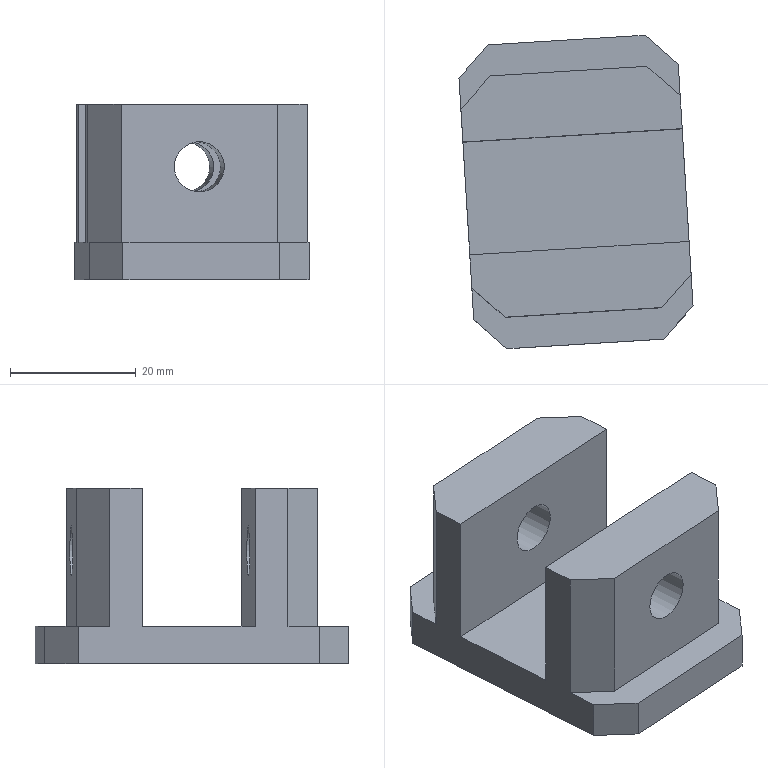Part | STEP file | 车灯-后视镜_id586_x_t | 1 solid | 24 faces | box 37.285 x 49.936 x 28 mm | volume 23540 mm3 | plane 22 | cylinder 2 | commonest cylinder face diameters 8 x2
STEP:
#1=CARTESIAN_POINT('',(116.538,2.661,-249.5));
#2=VERTEX_POINT('',#1);
#3=CARTESIAN_POINT('',(115.439,20.627,-249.5));
#4=VERTEX_POINT('',#3);
#5=CARTESIAN_POINT('',(117.102,-6.572,-249.5));
#6=DIRECTION('',(-0.06105,0.9981,0.));
#7=VECTOR('',#6,1.);
#8=LINE('',#5,#7);
#9=EDGE_CURVE('',#2,#4,#8,.T.);
#10=ORIENTED_EDGE('',*,*,#9,.T.);
#11=CARTESIAN_POINT('',(80.504,18.49,-249.5));
#12=VERTEX_POINT('',#11);
#13=CARTESIAN_POINT('',(103.493,19.896,-249.5));
#14=DIRECTION('',(0.9981,0.06105,0.));
#15=VECTOR('',#14,1.);
#16=LINE('',#13,#15);
#17=EDGE_CURVE('',#12,#4,#16,.T.);
#18=ORIENTED_EDGE('',*,*,#17,.F.);
#19=CARTESIAN_POINT('',(81.603,0.5239,-249.5));
#20=VERTEX_POINT('',#19);
#21=CARTESIAN_POINT('',(82.168,-8.709,-249.5));
#22=DIRECTION('',(0.06105,-0.9981,0.));
#23=VECTOR('',#22,1.);
#24=LINE('',#21,#23);
#25=EDGE_CURVE('',#12,#20,#24,.T.);
#26=ORIENTED_EDGE('',*,*,#25,.T.);
#27=CARTESIAN_POINT('',(104.591,1.93,-249.5));
#28=DIRECTION('',(-0.9981,-0.06105,0.));
#29=VECTOR('',#28,1.);
#30=LINE('',#27,#29);
#31=EDGE_CURVE('',#2,#20,#30,.T.);
#32=ORIENTED_EDGE('',*,*,#31,.F.);
#33=EDGE_LOOP('',(#10,#18,#26,#32));
#34=FACE_OUTER_BOUND('',#33,.T.);
#35=CARTESIAN_POINT('',(111.919,-6.889,-249.5));
#36=DIRECTION('',(0.,0.,1.));
#37=DIRECTION('',(-0.9981,-0.06105,0.));
#38=AXIS2_PLACEMENT_3D('',#35,#36,#37);
#39=PLANE('',#38);
#40=ADVANCED_FACE('',(#34),#39,.T.);
#41=CARTESIAN_POINT('',(117.163,-7.57,-249.5));
#42=VERTEX_POINT('',#41);
#43=CARTESIAN_POINT('',(116.858,-2.58,-249.5));
#44=VERTEX_POINT('',#43);
#45=CARTESIAN_POINT('',(116.4,4.906,-249.5));
#46=DIRECTION('',(-0.06105,0.9981,0.));
#47=VECTOR('',#46,1.);
#48=LINE('',#45,#47);
#49=EDGE_CURVE('',#42,#44,#48,.T.);
#50=ORIENTED_EDGE('',*,*,#49,.T.);
#51=CARTESIAN_POINT('',(112.173,-7.876,-249.5));
#52=VERTEX_POINT('',#51);
#53=CARTESIAN_POINT('',(116.858,-2.58,-249.5));
#54=DIRECTION('',(0.6626,0.749,0.));
#55=VECTOR('',#54,1.);
#56=LINE('',#53,#55);
#57=EDGE_CURVE('',#52,#44,#56,.T.);
#58=ORIENTED_EDGE('',*,*,#57,.F.);
#59=CARTESIAN_POINT('',(87.219,-9.402,-249.5));
#60=VERTEX_POINT('',#59);
#61=CARTESIAN_POINT('',(100.554,-8.586,-249.5));
#62=DIRECTION('',(0.9981,0.06105,0.));
#63=VECTOR('',#62,1.);
#64=LINE('',#61,#63);
#65=EDGE_CURVE('',#60,#52,#64,.T.);
#66=ORIENTED_EDGE('',*,*,#65,.F.);
#67=CARTESIAN_POINT('',(81.923,-4.716,-249.5));
#68=VERTEX_POINT('',#67);
#69=CARTESIAN_POINT('',(87.219,-9.402,-249.5));
#70=DIRECTION('',(0.749,-0.6626,0.));
#71=VECTOR('',#70,1.);
#72=LINE('',#69,#71);
#73=EDGE_CURVE('',#68,#60,#72,.T.);
#74=ORIENTED_EDGE('',*,*,#73,.F.);
#75=CARTESIAN_POINT('',(82.229,-9.707,-249.5));
#76=VERTEX_POINT('',#75);
#77=CARTESIAN_POINT('',(81.466,2.77,-249.5));
#78=DIRECTION('',(0.06105,-0.9981,0.));
#79=VECTOR('',#78,1.);
#80=LINE('',#77,#79);
#81=EDGE_CURVE('',#68,#76,#80,.T.);
#82=ORIENTED_EDGE('',*,*,#81,.T.);
#83=CARTESIAN_POINT('',(87.525,-14.392,-249.5));
#84=VERTEX_POINT('',#83);
#85=CARTESIAN_POINT('',(87.525,-14.392,-249.5));
#86=DIRECTION('',(-0.749,0.6626,0.));
#87=VECTOR('',#86,1.);
#88=LINE('',#85,#87);
#89=EDGE_CURVE('',#84,#76,#88,.T.);
#90=ORIENTED_EDGE('',*,*,#89,.F.);
#91=CARTESIAN_POINT('',(112.478,-12.866,-249.5));
#92=VERTEX_POINT('',#91);
#93=CARTESIAN_POINT('',(112.285,-12.878,-249.5));
#94=DIRECTION('',(0.9981,0.06105,0.));
#95=VECTOR('',#94,1.);
#96=LINE('',#93,#95);
#97=EDGE_CURVE('',#84,#92,#96,.T.);
#98=ORIENTED_EDGE('',*,*,#97,.T.);
#99=CARTESIAN_POINT('',(117.163,-7.57,-249.5));
#100=DIRECTION('',(-0.6626,-0.749,0.));
#101=VECTOR('',#100,1.);
#102=LINE('',#99,#101);
#103=EDGE_CURVE('',#42,#92,#102,.T.);
#104=ORIENTED_EDGE('',*,*,#103,.F.);
#105=EDGE_LOOP('',(#50,#58,#66,#74,#82,#90,#98,#104));
#106=FACE_OUTER_BOUND('',#105,.T.);
#107=CARTESIAN_POINT('',(111.217,4.589,-249.5));
#108=DIRECTION('',(0.,0.,1.));
#109=DIRECTION('',(-0.9981,-0.06105,0.));
#110=AXIS2_PLACEMENT_3D('',#107,#108,#109);
#111=PLANE('',#110);
#112=ADVANCED_FACE('',(#106),#111,.T.);
#113=CARTESIAN_POINT('',(109.517,35.543,-249.5));
#114=VERTEX_POINT('',#113);
#115=CARTESIAN_POINT('',(84.564,34.017,-249.5));
#116=VERTEX_POINT('',#115);
#117=CARTESIAN_POINT('',(109.324,35.532,-249.5));
#118=DIRECTION('',(-0.9981,-0.06105,0.));
#119=VECTOR('',#118,1.);
#120=LINE('',#117,#119);
#121=EDGE_CURVE('',#114,#116,#120,.T.);
#122=ORIENTED_EDGE('',*,*,#121,.T.);
#123=CARTESIAN_POINT('',(79.878,28.721,-249.5));
#124=VERTEX_POINT('',#123);
#125=CARTESIAN_POINT('',(79.878,28.721,-249.5));
#126=DIRECTION('',(0.6626,0.749,0.));
#127=VECTOR('',#126,1.);
#128=LINE('',#125,#127);
#129=EDGE_CURVE('',#124,#116,#128,.T.);
#130=ORIENTED_EDGE('',*,*,#129,.F.);
#131=CARTESIAN_POINT('',(80.184,23.73,-249.5));
#132=VERTEX_POINT('',#131);
#133=CARTESIAN_POINT('',(82.778,-18.69,-249.5));
#134=DIRECTION('',(0.06105,-0.9981,0.));
#135=VECTOR('',#134,1.);
#136=LINE('',#133,#135);
#137=EDGE_CURVE('',#124,#132,#136,.T.);
#138=ORIENTED_EDGE('',*,*,#137,.T.);
#139=CARTESIAN_POINT('',(84.869,29.026,-249.5));
#140=VERTEX_POINT('',#139);
#141=CARTESIAN_POINT('',(80.184,23.73,-249.5));
#142=DIRECTION('',(-0.6626,-0.749,0.));
#143=VECTOR('',#142,1.);
#144=LINE('',#141,#143);
#145=EDGE_CURVE('',#140,#132,#144,.T.);
#146=ORIENTED_EDGE('',*,*,#145,.F.);
#147=CARTESIAN_POINT('',(109.822,30.553,-249.5));
#148=VERTEX_POINT('',#147);
#149=CARTESIAN_POINT('',(98.204,29.842,-249.5));
#150=DIRECTION('',(-0.9981,-0.06105,0.));
#151=VECTOR('',#150,1.);
#152=LINE('',#149,#151);
#153=EDGE_CURVE('',#148,#140,#152,.T.);
#154=ORIENTED_EDGE('',*,*,#153,.F.);
#155=CARTESIAN_POINT('',(115.118,25.867,-249.5));
#156=VERTEX_POINT('',#155);
#157=CARTESIAN_POINT('',(109.822,30.553,-249.5));
#158=DIRECTION('',(-0.749,0.6626,0.));
#159=VECTOR('',#158,1.);
#160=LINE('',#157,#159);
#161=EDGE_CURVE('',#156,#148,#160,.T.);
#162=ORIENTED_EDGE('',*,*,#161,.F.);
#163=CARTESIAN_POINT('',(114.813,30.858,-249.5));
#164=VERTEX_POINT('',#163);
#165=CARTESIAN_POINT('',(117.713,-16.554,-249.5));
#166=DIRECTION('',(-0.06105,0.9981,0.));
#167=VECTOR('',#166,1.);
#168=LINE('',#165,#167);
#169=EDGE_CURVE('',#156,#164,#168,.T.);
#170=ORIENTED_EDGE('',*,*,#169,.T.);
#171=CARTESIAN_POINT('',(109.517,35.543,-249.5));
#172=DIRECTION('',(0.749,-0.6626,0.));
#173=VECTOR('',#172,1.);
#174=LINE('',#171,#173);
#175=EDGE_CURVE('',#114,#164,#174,.T.);
#176=ORIENTED_EDGE('',*,*,#175,.F.);
#177=EDGE_LOOP('',(#122,#130,#138,#146,#154,#162,#170,#176));
#178=FACE_OUTER_BOUND('',#177,.T.);
#179=CARTESIAN_POINT('',(112.529,-16.871,-249.5));
#180=DIRECTION('',(0.,0.,1.));
#181=DIRECTION('',(-0.9981,-0.06105,0.));
#182=AXIS2_PLACEMENT_3D('',#179,#180,#181);
#183=PLANE('',#182);
#184=ADVANCED_FACE('',(#178),#183,.T.);
#185=ORIENTED_EDGE('',*,*,#97,.F.);
#186=CARTESIAN_POINT('',(87.525,-14.392,-255.5));
#187=VERTEX_POINT('',#186);
#188=CARTESIAN_POINT('',(87.525,-14.392,-255.5));
#189=DIRECTION('',(0.,0.,1.));
#190=VECTOR('',#189,1.);
#191=LINE('',#188,#190);
#192=EDGE_CURVE('',#187,#84,#191,.T.);
#193=ORIENTED_EDGE('',*,*,#192,.F.);
#194=CARTESIAN_POINT('',(112.478,-12.866,-255.5));
#195=VERTEX_POINT('',#194);
#196=CARTESIAN_POINT('',(100.86,-13.577,-255.5));
#197=DIRECTION('',(-0.9981,-0.06105,0.));
#198=VECTOR('',#197,1.);
#199=LINE('',#196,#198);
#200=EDGE_CURVE('',#195,#187,#199,.T.);
#201=ORIENTED_EDGE('',*,*,#200,.F.);
#202=CARTESIAN_POINT('',(112.478,-12.866,-255.5));
#203=DIRECTION('',(0.,0.,-1.));
#204=VECTOR('',#203,1.);
#205=LINE('',#202,#204);
#206=EDGE_CURVE('',#92,#195,#205,.T.);
#207=ORIENTED_EDGE('',*,*,#206,.F.);
#208=EDGE_LOOP('',(#185,#193,#201,#207));
#209=FACE_OUTER_BOUND('',#208,.T.);
#210=CARTESIAN_POINT('',(100.86,-13.577,-255.5));
#211=DIRECTION('',(0.06105,-0.9981,0.));
#212=DIRECTION('',(0.,0.,-1.));
#213=AXIS2_PLACEMENT_3D('',#210,#211,#212);
#214=PLANE('',#213);
#215=ADVANCED_FACE('',(#209),#214,.T.);
#216=CARTESIAN_POINT('',(114.813,30.858,-255.5));
#217=VERTEX_POINT('',#216);
#218=CARTESIAN_POINT('',(117.163,-7.57,-255.5));
#219=VERTEX_POINT('',#218);
#220=CARTESIAN_POINT('',(115.271,23.372,-255.5));
#221=DIRECTION('',(0.06105,-0.9981,0.));
#222=VECTOR('',#221,1.);
#223=LINE('',#220,#222);
#224=EDGE_CURVE('',#217,#219,#223,.T.);
#225=ORIENTED_EDGE('',*,*,#224,.F.);
#226=CARTESIAN_POINT('',(114.813,30.858,-255.5));
#227=DIRECTION('',(0.,0.,-1.));
#228=VECTOR('',#227,1.);
#229=LINE('',#226,#228);
#230=EDGE_CURVE('',#164,#217,#229,.T.);
#231=ORIENTED_EDGE('',*,*,#230,.F.);
#232=ORIENTED_EDGE('',*,*,#169,.F.);
#233=CARTESIAN_POINT('',(115.118,25.867,-227.5));
#234=VERTEX_POINT('',#233);
#235=CARTESIAN_POINT('',(115.118,25.867,-255.5));
#236=DIRECTION('',(0.,0.,-1.));
#237=VECTOR('',#236,1.);
#238=LINE('',#235,#237);
#239=EDGE_CURVE('',#234,#156,#238,.T.);
#240=ORIENTED_EDGE('',*,*,#239,.F.);
#241=CARTESIAN_POINT('',(115.439,20.627,-227.5));
#242=VERTEX_POINT('',#241);
#243=CARTESIAN_POINT('',(115.454,20.377,-227.5));
#244=DIRECTION('',(-0.06105,0.9981,0.));
#245=VECTOR('',#244,1.);
#246=LINE('',#243,#245);
#247=EDGE_CURVE('',#242,#234,#246,.T.);
#248=ORIENTED_EDGE('',*,*,#247,.F.);
#249=CARTESIAN_POINT('',(115.439,20.627,-255.5));
#250=DIRECTION('',(0.,0.,-1.));
#251=VECTOR('',#250,1.);
#252=LINE('',#249,#251);
#253=EDGE_CURVE('',#242,#4,#252,.T.);
#254=ORIENTED_EDGE('',*,*,#253,.T.);
#255=ORIENTED_EDGE('',*,*,#9,.F.);
#256=CARTESIAN_POINT('',(116.538,2.661,-227.5));
#257=VERTEX_POINT('',#256);
#258=CARTESIAN_POINT('',(116.538,2.661,-243.));
#259=DIRECTION('',(0.,0.,-1.));
#260=VECTOR('',#259,1.);
#261=LINE('',#258,#260);
#262=EDGE_CURVE('',#257,#2,#261,.T.);
#263=ORIENTED_EDGE('',*,*,#262,.F.);
#264=CARTESIAN_POINT('',(116.858,-2.58,-227.5));
#265=VERTEX_POINT('',#264);
#266=CARTESIAN_POINT('',(114.996,27.863,-227.5));
#267=DIRECTION('',(-0.06105,0.9981,0.));
#268=VECTOR('',#267,1.);
#269=LINE('',#266,#268);
#270=EDGE_CURVE('',#265,#257,#269,.T.);
#271=ORIENTED_EDGE('',*,*,#270,.F.);
#272=CARTESIAN_POINT('',(116.858,-2.58,-255.5));
#273=DIRECTION('',(0.,0.,1.));
#274=VECTOR('',#273,1.);
#275=LINE('',#272,#274);
#276=EDGE_CURVE('',#44,#265,#275,.T.);
#277=ORIENTED_EDGE('',*,*,#276,.F.);
#278=ORIENTED_EDGE('',*,*,#49,.F.);
#279=CARTESIAN_POINT('',(117.163,-7.57,-255.5));
#280=DIRECTION('',(0.,0.,1.));
#281=VECTOR('',#280,1.);
#282=LINE('',#279,#281);
#283=EDGE_CURVE('',#219,#42,#282,.T.);
#284=ORIENTED_EDGE('',*,*,#283,.F.);
#285=EDGE_LOOP('',(#225,#231,#232,#240,#248,#254,#255,#263,#271,#277,#278,#284));
#286=FACE_OUTER_BOUND('',#285,.T.);
#287=CARTESIAN_POINT('',(115.271,23.372,-255.5));
#288=DIRECTION('',(0.9981,0.06105,0.));
#289=DIRECTION('',(0.,0.,1.));
#290=AXIS2_PLACEMENT_3D('',#287,#288,#289);
#291=PLANE('',#290);
#292=ADVANCED_FACE('',(#286),#291,.T.);
#293=CARTESIAN_POINT('',(84.564,34.017,-255.5));
#294=VERTEX_POINT('',#293);
#295=CARTESIAN_POINT('',(109.517,35.543,-255.5));
#296=VERTEX_POINT('',#295);
#297=CARTESIAN_POINT('',(97.899,34.833,-255.5));
#298=DIRECTION('',(0.9981,0.06105,0.));
#299=VECTOR('',#298,1.);
#300=LINE('',#297,#299);
#301=EDGE_CURVE('',#294,#296,#300,.T.);
#302=ORIENTED_EDGE('',*,*,#301,.F.);
#303=CARTESIAN_POINT('',(84.564,34.017,-255.5));
#304=DIRECTION('',(0.,0.,-1.));
#305=VECTOR('',#304,1.);
#306=LINE('',#303,#305);
#307=EDGE_CURVE('',#116,#294,#306,.T.);
#308=ORIENTED_EDGE('',*,*,#307,.F.);
#309=ORIENTED_EDGE('',*,*,#121,.F.);
#310=CARTESIAN_POINT('',(109.517,35.543,-255.5));
#311=DIRECTION('',(0.,0.,1.));
#312=VECTOR('',#311,1.);
#313=LINE('',#310,#312);
#314=EDGE_CURVE('',#296,#114,#313,.T.);
#315=ORIENTED_EDGE('',*,*,#314,.F.);
#316=EDGE_LOOP('',(#302,#308,#309,#315));
#317=FACE_OUTER_BOUND('',#316,.T.);
#318=CARTESIAN_POINT('',(97.899,34.833,-255.5));
#319=DIRECTION('',(-0.06105,0.9981,0.));
#320=DIRECTION('',(0.,0.,1.));
#321=AXIS2_PLACEMENT_3D('',#318,#319,#320);
#322=PLANE('',#321);
#323=ADVANCED_FACE('',(#317),#322,.T.);
#324=ORIENTED_EDGE('',*,*,#81,.F.);
#325=CARTESIAN_POINT('',(81.923,-4.716,-227.5));
#326=VERTEX_POINT('',#325);
#327=CARTESIAN_POINT('',(81.923,-4.716,-255.5));
#328=DIRECTION('',(0.,0.,-1.));
#329=VECTOR('',#328,1.);
#330=LINE('',#327,#329);
#331=EDGE_CURVE('',#326,#68,#330,.T.);
#332=ORIENTED_EDGE('',*,*,#331,.F.);
#333=CARTESIAN_POINT('',(81.603,0.5239,-227.5));
#334=VERTEX_POINT('',#333);
#335=CARTESIAN_POINT('',(80.061,25.727,-227.5));
#336=DIRECTION('',(0.06105,-0.9981,0.));
#337=VECTOR('',#336,1.);
#338=LINE('',#335,#337);
#339=EDGE_CURVE('',#334,#326,#338,.T.);
#340=ORIENTED_EDGE('',*,*,#339,.F.);
#341=CARTESIAN_POINT('',(81.603,0.5239,-243.));
#342=DIRECTION('',(0.,0.,1.));
#343=VECTOR('',#342,1.);
#344=LINE('',#341,#343);
#345=EDGE_CURVE('',#20,#334,#344,.T.);
#346=ORIENTED_EDGE('',*,*,#345,.F.);
#347=ORIENTED_EDGE('',*,*,#25,.F.);
#348=CARTESIAN_POINT('',(80.504,18.49,-227.5));
#349=VERTEX_POINT('',#348);
#350=CARTESIAN_POINT('',(80.504,18.49,-255.5));
#351=DIRECTION('',(0.,0.,1.));
#352=VECTOR('',#351,1.);
#353=LINE('',#350,#352);
#354=EDGE_CURVE('',#12,#349,#353,.T.);
#355=ORIENTED_EDGE('',*,*,#354,.T.);
#356=CARTESIAN_POINT('',(80.184,23.73,-227.5));
#357=VERTEX_POINT('',#356);
#358=CARTESIAN_POINT('',(80.519,18.241,-227.5));
#359=DIRECTION('',(0.06105,-0.9981,0.));
#360=VECTOR('',#359,1.);
#361=LINE('',#358,#360);
#362=EDGE_CURVE('',#357,#349,#361,.T.);
#363=ORIENTED_EDGE('',*,*,#362,.F.);
#364=CARTESIAN_POINT('',(80.184,23.73,-255.5));
#365=DIRECTION('',(0.,0.,1.));
#366=VECTOR('',#365,1.);
#367=LINE('',#364,#366);
#368=EDGE_CURVE('',#132,#357,#367,.T.);
#369=ORIENTED_EDGE('',*,*,#368,.F.);
#370=ORIENTED_EDGE('',*,*,#137,.F.);
#371=CARTESIAN_POINT('',(79.878,28.721,-255.5));
#372=VERTEX_POINT('',#371);
#373=CARTESIAN_POINT('',(79.878,28.721,-255.5));
#374=DIRECTION('',(0.,0.,1.));
#375=VECTOR('',#374,1.);
#376=LINE('',#373,#375);
#377=EDGE_CURVE('',#372,#124,#376,.T.);
#378=ORIENTED_EDGE('',*,*,#377,.F.);
#379=CARTESIAN_POINT('',(82.229,-9.707,-255.5));
#380=VERTEX_POINT('',#379);
#381=CARTESIAN_POINT('',(80.336,21.235,-255.5));
#382=DIRECTION('',(-0.06105,0.9981,0.));
#383=VECTOR('',#382,1.);
#384=LINE('',#381,#383);
#385=EDGE_CURVE('',#380,#372,#384,.T.);
#386=ORIENTED_EDGE('',*,*,#385,.F.);
#387=CARTESIAN_POINT('',(82.229,-9.707,-255.5));
#388=DIRECTION('',(0.,0.,-1.));
#389=VECTOR('',#388,1.);
#390=LINE('',#387,#389);
#391=EDGE_CURVE('',#76,#380,#390,.T.);
#392=ORIENTED_EDGE('',*,*,#391,.F.);
#393=EDGE_LOOP('',(#324,#332,#340,#346,#347,#355,#363,#369,#370,#378,#386,#392));
#394=FACE_OUTER_BOUND('',#393,.T.);
#395=CARTESIAN_POINT('',(80.336,21.235,-255.5));
#396=DIRECTION('',(-0.9981,-0.06105,0.));
#397=DIRECTION('',(0.,0.,-1.));
#398=AXIS2_PLACEMENT_3D('',#395,#396,#397);
#399=PLANE('',#398);
#400=ADVANCED_FACE('',(#394),#399,.T.);
#401=ORIENTED_EDGE('',*,*,#200,.T.);
#402=CARTESIAN_POINT('',(87.525,-14.392,-255.5));
#403=DIRECTION('',(0.749,-0.6626,0.));
#404=VECTOR('',#403,1.);
#405=LINE('',#402,#404);
#406=EDGE_CURVE('',#380,#187,#405,.T.);
#407=ORIENTED_EDGE('',*,*,#406,.F.);
#408=ORIENTED_EDGE('',*,*,#385,.T.);
#409=CARTESIAN_POINT('',(79.878,28.721,-255.5));
#410=DIRECTION('',(-0.6626,-0.749,0.));
#411=VECTOR('',#410,1.);
#412=LINE('',#409,#411);
#413=EDGE_CURVE('',#294,#372,#412,.T.);
#414=ORIENTED_EDGE('',*,*,#413,.F.);
#415=ORIENTED_EDGE('',*,*,#301,.T.);
#416=CARTESIAN_POINT('',(109.517,35.543,-255.5));
#417=DIRECTION('',(-0.749,0.6626,0.));
#418=VECTOR('',#417,1.);
#419=LINE('',#416,#418);
#420=EDGE_CURVE('',#217,#296,#419,.T.);
#421=ORIENTED_EDGE('',*,*,#420,.F.);
#422=ORIENTED_EDGE('',*,*,#224,.T.);
#423=CARTESIAN_POINT('',(117.163,-7.57,-255.5));
#424=DIRECTION('',(0.6626,0.749,0.));
#425=VECTOR('',#424,1.);
#426=LINE('',#423,#425);
#427=EDGE_CURVE('',#195,#219,#426,.T.);
#428=ORIENTED_EDGE('',*,*,#427,.F.);
#429=EDGE_LOOP('',(#401,#407,#408,#414,#415,#421,#422,#428));
#430=FACE_OUTER_BOUND('',#429,.T.);
#431=CARTESIAN_POINT('',(98.662,22.356,-255.5));
#432=DIRECTION('',(0.,0.,-1.));
#433=DIRECTION('',(0.9981,0.06105,0.));
#434=AXIS2_PLACEMENT_3D('',#431,#432,#433);
#435=PLANE('',#434);
#436=ADVANCED_FACE('',(#430),#435,.T.);
#437=CARTESIAN_POINT('',(93.353,29.545,-237.501));
#438=VERTEX_POINT('',#437);
#439=CARTESIAN_POINT('',(97.346,29.79,-237.501));
#440=DIRECTION('',(0.06105,-0.9981,0.));
#441=DIRECTION('',(-0.9981,-0.06105,0.));
#442=AXIS2_PLACEMENT_3D('',#439,#440,#441);
#443=CIRCLE('',#442,4.);
#444=EDGE_CURVE('',#438,#438,#443,.T.);
#445=ORIENTED_EDGE('',*,*,#444,.T.);
#446=EDGE_LOOP('',(#445));
#447=FACE_BOUND('',#446,.T.);
#448=ORIENTED_EDGE('',*,*,#153,.T.);
#449=CARTESIAN_POINT('',(84.869,29.026,-227.5));
#450=VERTEX_POINT('',#449);
#451=CARTESIAN_POINT('',(84.869,29.026,-255.5));
#452=DIRECTION('',(0.,0.,-1.));
#453=VECTOR('',#452,1.);
#454=LINE('',#451,#453);
#455=EDGE_CURVE('',#450,#140,#454,.T.);
#456=ORIENTED_EDGE('',*,*,#455,.F.);
#457=CARTESIAN_POINT('',(109.822,30.553,-227.5));
#458=VERTEX_POINT('',#457);
#459=CARTESIAN_POINT('',(98.204,29.842,-227.5));
#460=DIRECTION('',(-0.9981,-0.06105,0.));
#461=VECTOR('',#460,1.);
#462=LINE('',#459,#461);
#463=EDGE_CURVE('',#458,#450,#462,.T.);
#464=ORIENTED_EDGE('',*,*,#463,.F.);
#465=CARTESIAN_POINT('',(109.822,30.553,-255.5));
#466=DIRECTION('',(0.,0.,1.));
#467=VECTOR('',#466,1.);
#468=LINE('',#465,#467);
#469=EDGE_CURVE('',#148,#458,#468,.T.);
#470=ORIENTED_EDGE('',*,*,#469,.F.);
#471=EDGE_LOOP('',(#448,#456,#464,#470));
#472=FACE_BOUND('',#471,.T.);
#473=CARTESIAN_POINT('',(98.204,29.842,-255.5));
#474=DIRECTION('',(-0.06105,0.9981,0.));
#475=DIRECTION('',(0.,0.,1.));
#476=AXIS2_PLACEMENT_3D('',#473,#474,#475);
#477=PLANE('',#476);
#478=ADVANCED_FACE('',(#447,#472),#477,.T.);
#479=CARTESIAN_POINT('',(93.979,19.314,-237.501));
#480=VERTEX_POINT('',#479);
#481=CARTESIAN_POINT('',(97.971,19.559,-237.501));
#482=DIRECTION('',(0.06105,-0.9981,0.));
#483=DIRECTION('',(-0.9981,-0.06105,0.));
#484=AXIS2_PLACEMENT_3D('',#481,#482,#483);
#485=CIRCLE('',#484,4.);
#486=EDGE_CURVE('',#480,#480,#485,.T.);
#487=ORIENTED_EDGE('',*,*,#486,.F.);
#488=EDGE_LOOP('',(#487));
#489=FACE_BOUND('',#488,.T.);
#490=CARTESIAN_POINT('',(98.83,19.611,-227.5));
#491=DIRECTION('',(0.9981,0.06105,0.));
#492=VECTOR('',#491,1.);
#493=LINE('',#490,#492);
#494=EDGE_CURVE('',#349,#242,#493,.T.);
#495=ORIENTED_EDGE('',*,*,#494,.F.);
#496=ORIENTED_EDGE('',*,*,#354,.F.);
#497=ORIENTED_EDGE('',*,*,#17,.T.);
#498=ORIENTED_EDGE('',*,*,#253,.F.);
#499=EDGE_LOOP('',(#495,#496,#497,#498));
#500=FACE_BOUND('',#499,.T.);
#501=CARTESIAN_POINT('',(103.493,19.896,-243.));
#502=DIRECTION('',(-0.06105,0.9981,0.));
#503=DIRECTION('',(0.,0.,1.));
#504=AXIS2_PLACEMENT_3D('',#501,#502,#503);
#505=PLANE('',#504);
#506=ADVANCED_FACE('',(#489,#500),#505,.F.);
#507=ORIENTED_EDGE('',*,*,#463,.T.);
#508=CARTESIAN_POINT('',(80.184,23.73,-227.5));
#509=DIRECTION('',(0.6626,0.749,0.));
#510=VECTOR('',#509,1.);
#511=LINE('',#508,#510);
#512=EDGE_CURVE('',#357,#450,#511,.T.);
#513=ORIENTED_EDGE('',*,*,#512,.F.);
#514=ORIENTED_EDGE('',*,*,#362,.T.);
#515=ORIENTED_EDGE('',*,*,#494,.T.);
#516=ORIENTED_EDGE('',*,*,#247,.T.);
#517=CARTESIAN_POINT('',(109.822,30.553,-227.5));
#518=DIRECTION('',(0.749,-0.6626,0.));
#519=VECTOR('',#518,1.);
#520=LINE('',#517,#519);
#521=EDGE_CURVE('',#458,#234,#520,.T.);
#522=ORIENTED_EDGE('',*,*,#521,.F.);
#523=EDGE_LOOP('',(#507,#513,#514,#515,#516,#522));
#524=FACE_OUTER_BOUND('',#523,.T.);
#525=CARTESIAN_POINT('',(98.845,19.362,-227.5));
#526=DIRECTION('',(0.,0.,1.));
#527=DIRECTION('',(-0.9981,-0.06105,0.));
#528=AXIS2_PLACEMENT_3D('',#525,#526,#527);
#529=PLANE('',#528);
#530=ADVANCED_FACE('',(#524),#529,.T.);
#531=CARTESIAN_POINT('',(87.219,-9.402,-227.5));
#532=VERTEX_POINT('',#531);
#533=CARTESIAN_POINT('',(112.173,-7.876,-227.5));
#534=VERTEX_POINT('',#533);
#535=CARTESIAN_POINT('',(100.554,-8.586,-227.5));
#536=DIRECTION('',(0.9981,0.06105,0.));
#537=VECTOR('',#536,1.);
#538=LINE('',#535,#537);
#539=EDGE_CURVE('',#532,#534,#538,.T.);
#540=ORIENTED_EDGE('',*,*,#539,.T.);
#541=CARTESIAN_POINT('',(116.858,-2.58,-227.5));
#542=DIRECTION('',(-0.6626,-0.749,0.));
#543=VECTOR('',#542,1.);
#544=LINE('',#541,#543);
#545=EDGE_CURVE('',#265,#534,#544,.T.);
#546=ORIENTED_EDGE('',*,*,#545,.F.);
#547=ORIENTED_EDGE('',*,*,#270,.T.);
#548=CARTESIAN_POINT('',(104.591,1.93,-227.5));
#549=DIRECTION('',(0.9981,0.06105,0.));
#550=VECTOR('',#549,1.);
#551=LINE('',#548,#550);
#552=EDGE_CURVE('',#334,#257,#551,.T.);
#553=ORIENTED_EDGE('',*,*,#552,.F.);
#554=ORIENTED_EDGE('',*,*,#339,.T.);
#555=CARTESIAN_POINT('',(87.219,-9.402,-227.5));
#556=DIRECTION('',(-0.749,0.6626,0.));
#557=VECTOR('',#556,1.);
#558=LINE('',#555,#557);
#559=EDGE_CURVE('',#532,#326,#558,.T.);
#560=ORIENTED_EDGE('',*,*,#559,.F.);
#561=EDGE_LOOP('',(#540,#546,#547,#553,#554,#560));
#562=FACE_OUTER_BOUND('',#561,.T.);
#563=CARTESIAN_POINT('',(98.387,26.848,-227.5));
#564=DIRECTION('',(0.,0.,1.));
#565=DIRECTION('',(-0.9981,-0.06105,0.));
#566=AXIS2_PLACEMENT_3D('',#563,#564,#565);
#567=PLANE('',#566);
#568=ADVANCED_FACE('',(#562),#567,.T.);
#569=CARTESIAN_POINT('',(103.689,-8.394,-237.501));
#570=VERTEX_POINT('',#569);
#571=CARTESIAN_POINT('',(99.696,-8.639,-237.501));
#572=DIRECTION('',(-0.06105,0.9981,0.));
#573=DIRECTION('',(0.9981,0.06105,0.));
#574=AXIS2_PLACEMENT_3D('',#571,#572,#573);
#575=CIRCLE('',#574,4.);
#576=EDGE_CURVE('',#570,#570,#575,.T.);
#577=ORIENTED_EDGE('',*,*,#576,.T.);
#578=EDGE_LOOP('',(#577));
#579=FACE_BOUND('',#578,.T.);
#580=ORIENTED_EDGE('',*,*,#65,.T.);
#581=CARTESIAN_POINT('',(112.173,-7.876,-255.5));
#582=DIRECTION('',(0.,0.,-1.));
#583=VECTOR('',#582,1.);
#584=LINE('',#581,#583);
#585=EDGE_CURVE('',#534,#52,#584,.T.);
#586=ORIENTED_EDGE('',*,*,#585,.F.);
#587=ORIENTED_EDGE('',*,*,#539,.F.);
#588=CARTESIAN_POINT('',(87.219,-9.402,-255.5));
#589=DIRECTION('',(0.,0.,1.));
#590=VECTOR('',#589,1.);
#591=LINE('',#588,#590);
#592=EDGE_CURVE('',#60,#532,#591,.T.);
#593=ORIENTED_EDGE('',*,*,#592,.F.);
#594=EDGE_LOOP('',(#580,#586,#587,#593));
#595=FACE_BOUND('',#594,.T.);
#596=CARTESIAN_POINT('',(100.554,-8.586,-255.5));
#597=DIRECTION('',(0.06105,-0.9981,0.));
#598=DIRECTION('',(0.,0.,-1.));
#599=AXIS2_PLACEMENT_3D('',#596,#597,#598);
#600=PLANE('',#599);
#601=ADVANCED_FACE('',(#579,#595),#600,.T.);
#602=CARTESIAN_POINT('',(103.063,1.836,-237.501));
#603=VERTEX_POINT('',#602);
#604=CARTESIAN_POINT('',(99.07,1.592,-237.501));
#605=DIRECTION('',(-0.06105,0.9981,0.));
#606=DIRECTION('',(0.9981,0.06105,0.));
#607=AXIS2_PLACEMENT_3D('',#604,#605,#606);
#608=CIRCLE('',#607,4.);
#609=EDGE_CURVE('',#603,#603,#608,.T.);
#610=ORIENTED_EDGE('',*,*,#609,.F.);
#611=EDGE_LOOP('',(#610));
#612=FACE_BOUND('',#611,.T.);
#613=ORIENTED_EDGE('',*,*,#262,.T.);
#614=ORIENTED_EDGE('',*,*,#31,.T.);
#615=ORIENTED_EDGE('',*,*,#345,.T.);
#616=ORIENTED_EDGE('',*,*,#552,.T.);
#617=EDGE_LOOP('',(#613,#614,#615,#616));
#618=FACE_BOUND('',#617,.T.);
#619=CARTESIAN_POINT('',(104.591,1.93,-243.));
#620=DIRECTION('',(0.06105,-0.9981,0.));
#621=DIRECTION('',(0.,0.,-1.));
#622=AXIS2_PLACEMENT_3D('',#619,#620,#621);
#623=PLANE('',#622);
#624=ADVANCED_FACE('',(#612,#618),#623,.F.);
#625=ORIENTED_EDGE('',*,*,#576,.F.);
#626=EDGE_LOOP('',(#625));
#627=FACE_BOUND('',#626,.T.);
#628=ORIENTED_EDGE('',*,*,#609,.T.);
#629=EDGE_LOOP('',(#628));
#630=FACE_BOUND('',#629,.T.);
#631=CARTESIAN_POINT('',(101.003,-30.002,-237.501));
#632=DIRECTION('',(-0.06105,0.9981,0.));
#633=DIRECTION('',(0.,0.,1.));
#634=AXIS2_PLACEMENT_3D('',#631,#632,#633);
#635=CYLINDRICAL_SURFACE('',#634,4.);
#636=ADVANCED_FACE('',(#627,#630),#635,.F.);
#637=ORIENTED_EDGE('',*,*,#444,.F.);
#638=EDGE_LOOP('',(#637));
#639=FACE_BOUND('',#638,.T.);
#640=ORIENTED_EDGE('',*,*,#486,.T.);
#641=EDGE_LOOP('',(#640));
#642=FACE_BOUND('',#641,.T.);
#643=CARTESIAN_POINT('',(101.461,-37.488,-237.501));
#644=DIRECTION('',(-0.06105,0.9981,0.));
#645=DIRECTION('',(0.,0.,1.));
#646=AXIS2_PLACEMENT_3D('',#643,#644,#645);
#647=CYLINDRICAL_SURFACE('',#646,4.);
#648=ADVANCED_FACE('',(#639,#642),#647,.F.);
#649=ORIENTED_EDGE('',*,*,#161,.T.);
#650=ORIENTED_EDGE('',*,*,#469,.T.);
#651=ORIENTED_EDGE('',*,*,#521,.T.);
#652=ORIENTED_EDGE('',*,*,#239,.T.);
#653=EDGE_LOOP('',(#649,#650,#651,#652));
#654=FACE_OUTER_BOUND('',#653,.T.);
#655=CARTESIAN_POINT('',(109.822,30.553,-255.5));
#656=DIRECTION('',(-0.6626,-0.749,0.));
#657=DIRECTION('',(-0.749,0.6626,0.));
#658=AXIS2_PLACEMENT_3D('',#655,#656,#657);
#659=PLANE('',#658);
#660=ADVANCED_FACE('',(#654),#659,.F.);
#661=ORIENTED_EDGE('',*,*,#145,.T.);
#662=ORIENTED_EDGE('',*,*,#368,.T.);
#663=ORIENTED_EDGE('',*,*,#512,.T.);
#664=ORIENTED_EDGE('',*,*,#455,.T.);
#665=EDGE_LOOP('',(#661,#662,#663,#664));
#666=FACE_OUTER_BOUND('',#665,.T.);
#667=CARTESIAN_POINT('',(80.184,23.73,-255.5));
#668=DIRECTION('',(0.749,-0.6626,0.));
#669=DIRECTION('',(-0.6626,-0.749,0.));
#670=AXIS2_PLACEMENT_3D('',#667,#668,#669);
#671=PLANE('',#670);
#672=ADVANCED_FACE('',(#666),#671,.F.);
#673=ORIENTED_EDGE('',*,*,#73,.T.);
#674=ORIENTED_EDGE('',*,*,#592,.T.);
#675=ORIENTED_EDGE('',*,*,#559,.T.);
#676=ORIENTED_EDGE('',*,*,#331,.T.);
#677=EDGE_LOOP('',(#673,#674,#675,#676));
#678=FACE_OUTER_BOUND('',#677,.T.);
#679=CARTESIAN_POINT('',(87.219,-9.402,-255.5));
#680=DIRECTION('',(0.6626,0.749,0.));
#681=DIRECTION('',(0.749,-0.6626,0.));
#682=AXIS2_PLACEMENT_3D('',#679,#680,#681);
#683=PLANE('',#682);
#684=ADVANCED_FACE('',(#678),#683,.F.);
#685=ORIENTED_EDGE('',*,*,#57,.T.);
#686=ORIENTED_EDGE('',*,*,#276,.T.);
#687=ORIENTED_EDGE('',*,*,#545,.T.);
#688=ORIENTED_EDGE('',*,*,#585,.T.);
#689=EDGE_LOOP('',(#685,#686,#687,#688));
#690=FACE_OUTER_BOUND('',#689,.T.);
#691=CARTESIAN_POINT('',(116.858,-2.58,-255.5));
#692=DIRECTION('',(-0.749,0.6626,0.));
#693=DIRECTION('',(0.6626,0.749,0.));
#694=AXIS2_PLACEMENT_3D('',#691,#692,#693);
#695=PLANE('',#694);
#696=ADVANCED_FACE('',(#690),#695,.F.);
#697=ORIENTED_EDGE('',*,*,#427,.T.);
#698=ORIENTED_EDGE('',*,*,#283,.T.);
#699=ORIENTED_EDGE('',*,*,#103,.T.);
#700=ORIENTED_EDGE('',*,*,#206,.T.);
#701=EDGE_LOOP('',(#697,#698,#699,#700));
#702=FACE_OUTER_BOUND('',#701,.T.);
#703=CARTESIAN_POINT('',(117.163,-7.57,-255.5));
#704=DIRECTION('',(-0.749,0.6626,0.));
#705=DIRECTION('',(0.6626,0.749,0.));
#706=AXIS2_PLACEMENT_3D('',#703,#704,#705);
#707=PLANE('',#706);
#708=ADVANCED_FACE('',(#702),#707,.F.);
#709=ORIENTED_EDGE('',*,*,#406,.T.);
#710=ORIENTED_EDGE('',*,*,#192,.T.);
#711=ORIENTED_EDGE('',*,*,#89,.T.);
#712=ORIENTED_EDGE('',*,*,#391,.T.);
#713=EDGE_LOOP('',(#709,#710,#711,#712));
#714=FACE_OUTER_BOUND('',#713,.T.);
#715=CARTESIAN_POINT('',(87.525,-14.392,-255.5));
#716=DIRECTION('',(0.6626,0.749,0.));
#717=DIRECTION('',(0.749,-0.6626,0.));
#718=AXIS2_PLACEMENT_3D('',#715,#716,#717);
#719=PLANE('',#718);
#720=ADVANCED_FACE('',(#714),#719,.F.);
#721=ORIENTED_EDGE('',*,*,#420,.T.);
#722=ORIENTED_EDGE('',*,*,#314,.T.);
#723=ORIENTED_EDGE('',*,*,#175,.T.);
#724=ORIENTED_EDGE('',*,*,#230,.T.);
#725=EDGE_LOOP('',(#721,#722,#723,#724));
#726=FACE_OUTER_BOUND('',#725,.T.);
#727=CARTESIAN_POINT('',(109.517,35.543,-255.5));
#728=DIRECTION('',(-0.6626,-0.749,0.));
#729=DIRECTION('',(-0.749,0.6626,0.));
#730=AXIS2_PLACEMENT_3D('',#727,#728,#729);
#731=PLANE('',#730);
#732=ADVANCED_FACE('',(#726),#731,.F.);
#733=ORIENTED_EDGE('',*,*,#413,.T.);
#734=ORIENTED_EDGE('',*,*,#377,.T.);
#735=ORIENTED_EDGE('',*,*,#129,.T.);
#736=ORIENTED_EDGE('',*,*,#307,.T.);
#737=EDGE_LOOP('',(#733,#734,#735,#736));
#738=FACE_OUTER_BOUND('',#737,.T.);
#739=CARTESIAN_POINT('',(79.878,28.721,-255.5));
#740=DIRECTION('',(0.749,-0.6626,0.));
#741=DIRECTION('',(-0.6626,-0.749,0.));
#742=AXIS2_PLACEMENT_3D('',#739,#740,#741);
#743=PLANE('',#742);
#744=ADVANCED_FACE('',(#738),#743,.F.);
#745=CLOSED_SHELL('',(#40,#112,#184,#215,#292,#323,#400,#436,#478,#506,#530,#568,#601,#624,#636,#648,#660,#672,#684,#696,#708,#720,#732,#744));
#746=MANIFOLD_SOLID_BREP('',#745);
#747=(LENGTH_UNIT()NAMED_UNIT(*)SI_UNIT(.MILLI.,.METRE.));
#748=UNCERTAINTY_MEASURE_WITH_UNIT(LENGTH_MEASURE(0.00002),#747,'','');
#749=(NAMED_UNIT(*)PLANE_ANGLE_UNIT()SI_UNIT($,.RADIAN.));
#750=PLANE_ANGLE_MEASURE_WITH_UNIT(PLANE_ANGLE_MEASURE(0.01745),#749);
#751=DIMENSIONAL_EXPONENTS(0.,0.,0.,0.,0.,0.,0.);
#752=(CONVERSION_BASED_UNIT('DEGREE',#750)NAMED_UNIT(#751)PLANE_ANGLE_UNIT());
#753=(NAMED_UNIT(*)SI_UNIT($,.STERADIAN.)SOLID_ANGLE_UNIT());
#754=(GEOMETRIC_REPRESENTATION_CONTEXT(3)GLOBAL_UNCERTAINTY_ASSIGNED_CONTEXT((#748))GLOBAL_UNIT_ASSIGNED_CONTEXT((#747,#752,#753))REPRESENTATION_CONTEXT('',''));
#755=ADVANCED_BREP_SHAPE_REPRESENTATION('',(#746),#754);